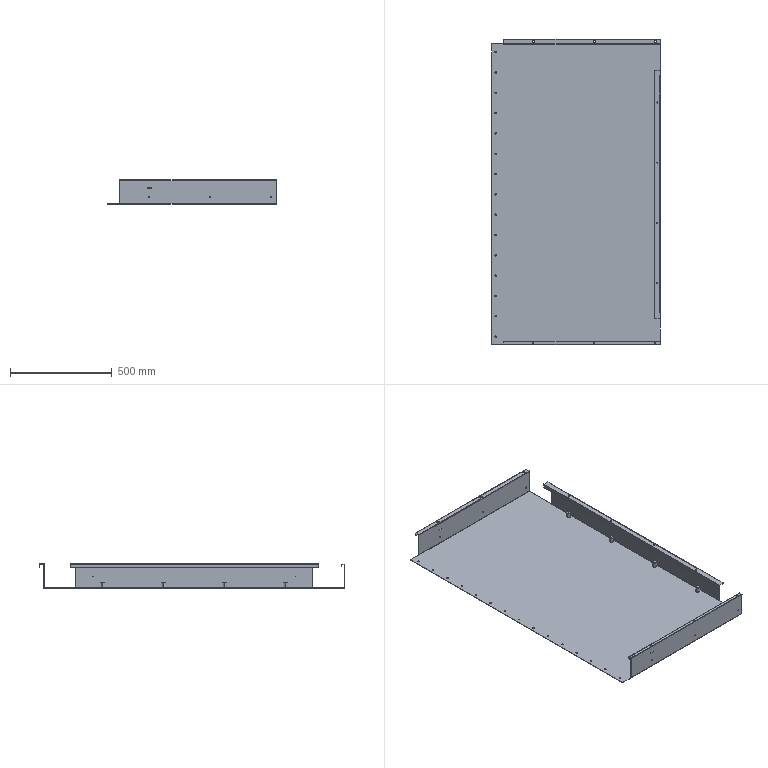Part | STEP file | SX-004-01 | 1 solid | 216 faces | box 830.5 x 1503 x 122 mm | volume 3328995 mm3 | cylinder 108 | plane 100 | cone 8 | commonest cylinder face diameters 7 x30 5.4 x26 0.4 x9 4.4 x9 8.5 x8 12.5 x8